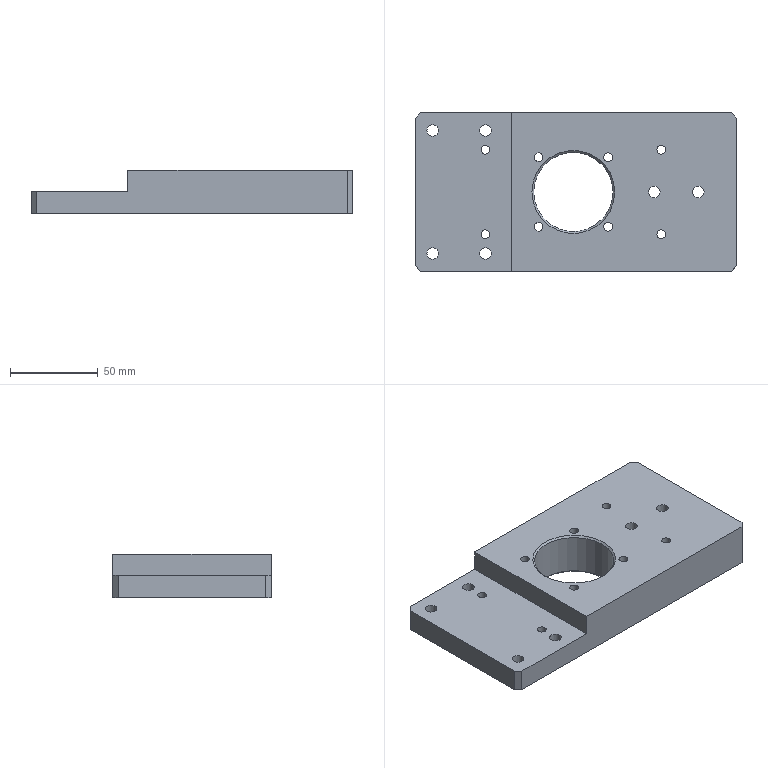Part | 1 solid | 47 faces | box 183 x 90 x 25 mm | volume 301566 mm3 | cylinder 24 | plane 18 | cone 5 | commonest cylinder face diameters 5 x11 6.6 x6 11 x6 45.1 x1
STEP:
#1=CARTESIAN_POINT('',(39.,0.,-5.7));
#2=VERTEX_POINT('',#1);
#3=CARTESIAN_POINT('',(44.5,0.,-5.7));
#4=DIRECTION('',(0.,0.,-1.));
#5=DIRECTION('',(-1.,0.,0.));
#6=AXIS2_PLACEMENT_3D('',#3,#4,#5);
#7=CIRCLE('',#6,5.5);
#8=EDGE_CURVE('',#2,#2,#7,.T.);
#9=ORIENTED_EDGE('',*,*,#8,.T.);
#10=EDGE_LOOP('',(#9));
#11=FACE_BOUND('',#10,.T.);
#12=CARTESIAN_POINT('',(41.2,0.,-5.7));
#13=VERTEX_POINT('',#12);
#14=CARTESIAN_POINT('',(44.5,0.,-5.7));
#15=DIRECTION('',(0.,0.,-1.));
#16=DIRECTION('',(-1.,0.,0.));
#17=AXIS2_PLACEMENT_3D('',#14,#15,#16);
#18=CIRCLE('',#17,3.3);
#19=EDGE_CURVE('',#13,#13,#18,.T.);
#20=ORIENTED_EDGE('',*,*,#19,.F.);
#21=EDGE_LOOP('',(#20));
#22=FACE_BOUND('',#21,.T.);
#23=CARTESIAN_POINT('',(47.8,0.,-5.7));
#24=DIRECTION('',(0.,0.,1.));
#25=DIRECTION('',(1.,0.,0.));
#26=AXIS2_PLACEMENT_3D('',#23,#24,#25);
#27=PLANE('',#26);
#28=ADVANCED_FACE('',(#11,#22),#27,.F.);
#29=CARTESIAN_POINT('',(75.,0.,-5.7));
#30=VERTEX_POINT('',#29);
#31=CARTESIAN_POINT('',(69.5,0.,-5.7));
#32=DIRECTION('',(0.,0.,-1.));
#33=DIRECTION('',(1.,0.,0.));
#34=AXIS2_PLACEMENT_3D('',#31,#32,#33);
#35=CIRCLE('',#34,5.5);
#36=EDGE_CURVE('',#30,#30,#35,.T.);
#37=ORIENTED_EDGE('',*,*,#36,.T.);
#38=EDGE_LOOP('',(#37));
#39=FACE_BOUND('',#38,.T.);
#40=CARTESIAN_POINT('',(72.8,0.,-5.7));
#41=VERTEX_POINT('',#40);
#42=CARTESIAN_POINT('',(69.5,0.,-5.7));
#43=DIRECTION('',(0.,0.,-1.));
#44=DIRECTION('',(1.,0.,0.));
#45=AXIS2_PLACEMENT_3D('',#42,#43,#44);
#46=CIRCLE('',#45,3.3);
#47=EDGE_CURVE('',#41,#41,#46,.T.);
#48=ORIENTED_EDGE('',*,*,#47,.F.);
#49=EDGE_LOOP('',(#48));
#50=FACE_BOUND('',#49,.T.);
#51=CARTESIAN_POINT('',(47.8,0.,-5.7));
#52=DIRECTION('',(0.,0.,1.));
#53=DIRECTION('',(1.,0.,0.));
#54=AXIS2_PLACEMENT_3D('',#51,#52,#53);
#55=PLANE('',#54);
#56=ADVANCED_FACE('',(#39,#50),#55,.F.);
#57=CARTESIAN_POINT('',(-88.5,45.,0.5));
#58=VERTEX_POINT('',#57);
#59=CARTESIAN_POINT('',(-91.5,42.,0.5));
#60=VERTEX_POINT('',#59);
#61=CARTESIAN_POINT('',(-91.5,42.,0.5));
#62=DIRECTION('',(-0.7071,-0.7071,0.));
#63=VECTOR('',#62,1000.);
#64=LINE('',#61,#63);
#65=EDGE_CURVE('',#58,#60,#64,.T.);
#66=ORIENTED_EDGE('',*,*,#65,.F.);
#67=CARTESIAN_POINT('',(-88.5,45.,-12.5));
#68=VERTEX_POINT('',#67);
#69=CARTESIAN_POINT('',(-88.5,45.,12.5));
#70=DIRECTION('',(0.,0.,1.));
#71=VECTOR('',#70,1000.);
#72=LINE('',#69,#71);
#73=EDGE_CURVE('',#68,#58,#72,.T.);
#74=ORIENTED_EDGE('',*,*,#73,.F.);
#75=CARTESIAN_POINT('',(-91.5,42.,-12.5));
#76=VERTEX_POINT('',#75);
#77=CARTESIAN_POINT('',(-91.5,42.,-12.5));
#78=DIRECTION('',(0.7071,0.7071,0.));
#79=VECTOR('',#78,1000.);
#80=LINE('',#77,#79);
#81=EDGE_CURVE('',#76,#68,#80,.T.);
#82=ORIENTED_EDGE('',*,*,#81,.F.);
#83=CARTESIAN_POINT('',(-91.5,42.,12.5));
#84=DIRECTION('',(0.,0.,-1.));
#85=VECTOR('',#84,1000.);
#86=LINE('',#83,#85);
#87=EDGE_CURVE('',#60,#76,#86,.T.);
#88=ORIENTED_EDGE('',*,*,#87,.F.);
#89=EDGE_LOOP('',(#66,#74,#82,#88));
#90=FACE_BOUND('',#89,.T.);
#91=CARTESIAN_POINT('',(-91.5,42.,12.5));
#92=DIRECTION('',(0.7071,-0.7071,0.));
#93=DIRECTION('',(0.,0.,-1.));
#94=AXIS2_PLACEMENT_3D('',#91,#92,#93);
#95=PLANE('',#94);
#96=ADVANCED_FACE('',(#90),#95,.F.);
#97=CARTESIAN_POINT('',(91.5,42.,12.5));
#98=VERTEX_POINT('',#97);
#99=CARTESIAN_POINT('',(88.5,45.,12.5));
#100=VERTEX_POINT('',#99);
#101=CARTESIAN_POINT('',(66.75,66.75,12.5));
#102=DIRECTION('',(-0.7071,0.7071,0.));
#103=VECTOR('',#102,1000.);
#104=LINE('',#101,#103);
#105=EDGE_CURVE('',#98,#100,#104,.T.);
#106=ORIENTED_EDGE('',*,*,#105,.F.);
#107=CARTESIAN_POINT('',(91.5,42.,-12.5));
#108=VERTEX_POINT('',#107);
#109=CARTESIAN_POINT('',(91.5,42.,12.5));
#110=DIRECTION('',(0.,0.,1.));
#111=VECTOR('',#110,1000.);
#112=LINE('',#109,#111);
#113=EDGE_CURVE('',#108,#98,#112,.T.);
#114=ORIENTED_EDGE('',*,*,#113,.F.);
#115=CARTESIAN_POINT('',(88.5,45.,-12.5));
#116=VERTEX_POINT('',#115);
#117=CARTESIAN_POINT('',(88.5,45.,-12.5));
#118=DIRECTION('',(0.7071,-0.7071,0.));
#119=VECTOR('',#118,1000.);
#120=LINE('',#117,#119);
#121=EDGE_CURVE('',#116,#108,#120,.T.);
#122=ORIENTED_EDGE('',*,*,#121,.F.);
#123=CARTESIAN_POINT('',(88.5,45.,12.5));
#124=DIRECTION('',(0.,0.,-1.));
#125=VECTOR('',#124,1000.);
#126=LINE('',#123,#125);
#127=EDGE_CURVE('',#100,#116,#126,.T.);
#128=ORIENTED_EDGE('',*,*,#127,.F.);
#129=EDGE_LOOP('',(#106,#114,#122,#128));
#130=FACE_BOUND('',#129,.T.);
#131=CARTESIAN_POINT('',(88.5,45.,12.5));
#132=DIRECTION('',(-0.7071,-0.7071,0.));
#133=DIRECTION('',(0.,0.,-1.));
#134=AXIS2_PLACEMENT_3D('',#131,#132,#133);
#135=PLANE('',#134);
#136=ADVANCED_FACE('',(#130),#135,.F.);
#137=CARTESIAN_POINT('',(88.5,-45.,12.5));
#138=VERTEX_POINT('',#137);
#139=CARTESIAN_POINT('',(91.5,-42.,12.5));
#140=VERTEX_POINT('',#139);
#141=CARTESIAN_POINT('',(66.75,-66.75,12.5));
#142=DIRECTION('',(0.7071,0.7071,0.));
#143=VECTOR('',#142,1000.);
#144=LINE('',#141,#143);
#145=EDGE_CURVE('',#138,#140,#144,.T.);
#146=ORIENTED_EDGE('',*,*,#145,.F.);
#147=CARTESIAN_POINT('',(88.5,-45.,-12.5));
#148=VERTEX_POINT('',#147);
#149=CARTESIAN_POINT('',(88.5,-45.,12.5));
#150=DIRECTION('',(0.,0.,1.));
#151=VECTOR('',#150,1000.);
#152=LINE('',#149,#151);
#153=EDGE_CURVE('',#148,#138,#152,.T.);
#154=ORIENTED_EDGE('',*,*,#153,.F.);
#155=CARTESIAN_POINT('',(91.5,-42.,-12.5));
#156=VERTEX_POINT('',#155);
#157=CARTESIAN_POINT('',(91.5,-42.,-12.5));
#158=DIRECTION('',(-0.7071,-0.7071,0.));
#159=VECTOR('',#158,1000.);
#160=LINE('',#157,#159);
#161=EDGE_CURVE('',#156,#148,#160,.T.);
#162=ORIENTED_EDGE('',*,*,#161,.F.);
#163=CARTESIAN_POINT('',(91.5,-42.,12.5));
#164=DIRECTION('',(0.,0.,-1.));
#165=VECTOR('',#164,1000.);
#166=LINE('',#163,#165);
#167=EDGE_CURVE('',#140,#156,#166,.T.);
#168=ORIENTED_EDGE('',*,*,#167,.F.);
#169=EDGE_LOOP('',(#146,#154,#162,#168));
#170=FACE_BOUND('',#169,.T.);
#171=CARTESIAN_POINT('',(91.5,-42.,12.5));
#172=DIRECTION('',(-0.7071,0.7071,0.));
#173=DIRECTION('',(0.,0.,-1.));
#174=AXIS2_PLACEMENT_3D('',#171,#172,#173);
#175=PLANE('',#174);
#176=ADVANCED_FACE('',(#170),#175,.F.);
#177=CARTESIAN_POINT('',(-91.5,-42.,0.5));
#178=VERTEX_POINT('',#177);
#179=CARTESIAN_POINT('',(-88.5,-45.,0.5));
#180=VERTEX_POINT('',#179);
#181=CARTESIAN_POINT('',(-88.5,-45.,0.5));
#182=DIRECTION('',(0.7071,-0.7071,0.));
#183=VECTOR('',#182,1000.);
#184=LINE('',#181,#183);
#185=EDGE_CURVE('',#178,#180,#184,.T.);
#186=ORIENTED_EDGE('',*,*,#185,.F.);
#187=CARTESIAN_POINT('',(-91.5,-42.,-12.5));
#188=VERTEX_POINT('',#187);
#189=CARTESIAN_POINT('',(-91.5,-42.,12.5));
#190=DIRECTION('',(0.,0.,1.));
#191=VECTOR('',#190,1000.);
#192=LINE('',#189,#191);
#193=EDGE_CURVE('',#188,#178,#192,.T.);
#194=ORIENTED_EDGE('',*,*,#193,.F.);
#195=CARTESIAN_POINT('',(-88.5,-45.,-12.5));
#196=VERTEX_POINT('',#195);
#197=CARTESIAN_POINT('',(-88.5,-45.,-12.5));
#198=DIRECTION('',(-0.7071,0.7071,0.));
#199=VECTOR('',#198,1000.);
#200=LINE('',#197,#199);
#201=EDGE_CURVE('',#196,#188,#200,.T.);
#202=ORIENTED_EDGE('',*,*,#201,.F.);
#203=CARTESIAN_POINT('',(-88.5,-45.,12.5));
#204=DIRECTION('',(0.,0.,-1.));
#205=VECTOR('',#204,1000.);
#206=LINE('',#203,#205);
#207=EDGE_CURVE('',#180,#196,#206,.T.);
#208=ORIENTED_EDGE('',*,*,#207,.F.);
#209=EDGE_LOOP('',(#186,#194,#202,#208));
#210=FACE_BOUND('',#209,.T.);
#211=CARTESIAN_POINT('',(-88.5,-45.,12.5));
#212=DIRECTION('',(0.7071,0.7071,0.));
#213=DIRECTION('',(0.,0.,-1.));
#214=AXIS2_PLACEMENT_3D('',#211,#212,#213);
#215=PLANE('',#214);
#216=ADVANCED_FACE('',(#210),#215,.F.);
#217=CARTESIAN_POINT('',(-76.,35.,-6.1));
#218=VERTEX_POINT('',#217);
#219=CARTESIAN_POINT('',(-81.5,35.,-6.1));
#220=DIRECTION('',(0.,0.,-1.));
#221=DIRECTION('',(1.,0.,0.));
#222=AXIS2_PLACEMENT_3D('',#219,#220,#221);
#223=CIRCLE('',#222,5.5);
#224=EDGE_CURVE('',#218,#218,#223,.T.);
#225=ORIENTED_EDGE('',*,*,#224,.T.);
#226=EDGE_LOOP('',(#225));
#227=FACE_BOUND('',#226,.T.);
#228=CARTESIAN_POINT('',(-78.2,35.,-6.1));
#229=VERTEX_POINT('',#228);
#230=CARTESIAN_POINT('',(-81.5,35.,-6.1));
#231=DIRECTION('',(0.,0.,-1.));
#232=DIRECTION('',(1.,0.,0.));
#233=AXIS2_PLACEMENT_3D('',#230,#231,#232);
#234=CIRCLE('',#233,3.3);
#235=EDGE_CURVE('',#229,#229,#234,.T.);
#236=ORIENTED_EDGE('',*,*,#235,.F.);
#237=EDGE_LOOP('',(#236));
#238=FACE_BOUND('',#237,.T.);
#239=CARTESIAN_POINT('',(-48.2,35.,-6.1));
#240=DIRECTION('',(0.,0.,1.));
#241=DIRECTION('',(1.,0.,0.));
#242=AXIS2_PLACEMENT_3D('',#239,#240,#241);
#243=PLANE('',#242);
#244=ADVANCED_FACE('',(#227,#238),#243,.F.);
#245=CARTESIAN_POINT('',(-57.,35.,-6.1));
#246=VERTEX_POINT('',#245);
#247=CARTESIAN_POINT('',(-51.5,35.,-6.1));
#248=DIRECTION('',(0.,0.,-1.));
#249=DIRECTION('',(-1.,0.,0.));
#250=AXIS2_PLACEMENT_3D('',#247,#248,#249);
#251=CIRCLE('',#250,5.5);
#252=EDGE_CURVE('',#246,#246,#251,.T.);
#253=ORIENTED_EDGE('',*,*,#252,.T.);
#254=EDGE_LOOP('',(#253));
#255=FACE_BOUND('',#254,.T.);
#256=CARTESIAN_POINT('',(-54.8,35.,-6.1));
#257=VERTEX_POINT('',#256);
#258=CARTESIAN_POINT('',(-51.5,35.,-6.1));
#259=DIRECTION('',(0.,0.,-1.));
#260=DIRECTION('',(-1.,0.,0.));
#261=AXIS2_PLACEMENT_3D('',#258,#259,#260);
#262=CIRCLE('',#261,3.3);
#263=EDGE_CURVE('',#257,#257,#262,.T.);
#264=ORIENTED_EDGE('',*,*,#263,.F.);
#265=EDGE_LOOP('',(#264));
#266=FACE_BOUND('',#265,.T.);
#267=CARTESIAN_POINT('',(-48.2,35.,-6.1));
#268=DIRECTION('',(0.,0.,1.));
#269=DIRECTION('',(1.,0.,0.));
#270=AXIS2_PLACEMENT_3D('',#267,#268,#269);
#271=PLANE('',#270);
#272=ADVANCED_FACE('',(#255,#266),#271,.F.);
#273=CARTESIAN_POINT('',(-46.,-35.,-6.1));
#274=VERTEX_POINT('',#273);
#275=CARTESIAN_POINT('',(-51.5,-35.,-6.1));
#276=DIRECTION('',(0.,0.,-1.));
#277=DIRECTION('',(1.,0.,0.));
#278=AXIS2_PLACEMENT_3D('',#275,#276,#277);
#279=CIRCLE('',#278,5.5);
#280=EDGE_CURVE('',#274,#274,#279,.T.);
#281=ORIENTED_EDGE('',*,*,#280,.T.);
#282=EDGE_LOOP('',(#281));
#283=FACE_BOUND('',#282,.T.);
#284=CARTESIAN_POINT('',(-48.2,-35.,-6.1));
#285=VERTEX_POINT('',#284);
#286=CARTESIAN_POINT('',(-51.5,-35.,-6.1));
#287=DIRECTION('',(0.,0.,-1.));
#288=DIRECTION('',(1.,0.,0.));
#289=AXIS2_PLACEMENT_3D('',#286,#287,#288);
#290=CIRCLE('',#289,3.3);
#291=EDGE_CURVE('',#285,#285,#290,.T.);
#292=ORIENTED_EDGE('',*,*,#291,.F.);
#293=EDGE_LOOP('',(#292));
#294=FACE_BOUND('',#293,.T.);
#295=CARTESIAN_POINT('',(-48.2,35.,-6.1));
#296=DIRECTION('',(0.,0.,1.));
#297=DIRECTION('',(1.,0.,0.));
#298=AXIS2_PLACEMENT_3D('',#295,#296,#297);
#299=PLANE('',#298);
#300=ADVANCED_FACE('',(#283,#294),#299,.F.);
#301=CARTESIAN_POINT('',(-76.,-35.,-6.1));
#302=VERTEX_POINT('',#301);
#303=CARTESIAN_POINT('',(-81.5,-35.,-6.1));
#304=DIRECTION('',(0.,0.,-1.));
#305=DIRECTION('',(1.,0.,0.));
#306=AXIS2_PLACEMENT_3D('',#303,#304,#305);
#307=CIRCLE('',#306,5.5);
#308=EDGE_CURVE('',#302,#302,#307,.T.);
#309=ORIENTED_EDGE('',*,*,#308,.T.);
#310=EDGE_LOOP('',(#309));
#311=FACE_BOUND('',#310,.T.);
#312=CARTESIAN_POINT('',(-78.2,-35.,-6.1));
#313=VERTEX_POINT('',#312);
#314=CARTESIAN_POINT('',(-81.5,-35.,-6.1));
#315=DIRECTION('',(0.,0.,-1.));
#316=DIRECTION('',(1.,0.,0.));
#317=AXIS2_PLACEMENT_3D('',#314,#315,#316);
#318=CIRCLE('',#317,3.3);
#319=EDGE_CURVE('',#313,#313,#318,.T.);
#320=ORIENTED_EDGE('',*,*,#319,.F.);
#321=EDGE_LOOP('',(#320));
#322=FACE_BOUND('',#321,.T.);
#323=CARTESIAN_POINT('',(-48.2,35.,-6.1));
#324=DIRECTION('',(0.,0.,1.));
#325=DIRECTION('',(1.,0.,0.));
#326=AXIS2_PLACEMENT_3D('',#323,#324,#325);
#327=PLANE('',#326);
#328=ADVANCED_FACE('',(#311,#322),#327,.F.);
#329=CARTESIAN_POINT('',(-91.5,-45.,0.5));
#330=DIRECTION('',(0.,-1.,0.));
#331=VECTOR('',#330,1000.);
#332=LINE('',#329,#331);
#333=EDGE_CURVE('',#60,#178,#332,.T.);
#334=ORIENTED_EDGE('',*,*,#333,.T.);
#335=ORIENTED_EDGE('',*,*,#185,.T.);
#336=CARTESIAN_POINT('',(-36.5,-45.,0.5));
#337=VERTEX_POINT('',#336);
#338=CARTESIAN_POINT('',(-91.5,-45.,0.5));
#339=DIRECTION('',(1.,0.,0.));
#340=VECTOR('',#339,1000.);
#341=LINE('',#338,#340);
#342=EDGE_CURVE('',#180,#337,#341,.T.);
#343=ORIENTED_EDGE('',*,*,#342,.T.);
#344=CARTESIAN_POINT('',(-36.5,45.,0.5));
#345=VERTEX_POINT('',#344);
#346=CARTESIAN_POINT('',(-36.5,-45.,0.5));
#347=DIRECTION('',(0.,1.,0.));
#348=VECTOR('',#347,1000.);
#349=LINE('',#346,#348);
#350=EDGE_CURVE('',#337,#345,#349,.T.);
#351=ORIENTED_EDGE('',*,*,#350,.T.);
#352=CARTESIAN_POINT('',(-91.5,45.,0.5));
#353=DIRECTION('',(-1.,0.,0.));
#354=VECTOR('',#353,1000.);
#355=LINE('',#352,#354);
#356=EDGE_CURVE('',#345,#58,#355,.T.);
#357=ORIENTED_EDGE('',*,*,#356,.T.);
#358=ORIENTED_EDGE('',*,*,#65,.T.);
#359=EDGE_LOOP('',(#334,#335,#343,#351,#357,#358));
#360=FACE_BOUND('',#359,.T.);
#361=CARTESIAN_POINT('',(-84.8,-35.,0.5));
#362=VERTEX_POINT('',#361);
#363=CARTESIAN_POINT('',(-81.5,-35.,0.5));
#364=DIRECTION('',(0.,0.,-1.));
#365=DIRECTION('',(-1.,0.,0.));
#366=AXIS2_PLACEMENT_3D('',#363,#364,#365);
#367=CIRCLE('',#366,3.3);
#368=EDGE_CURVE('',#362,#362,#367,.T.);
#369=ORIENTED_EDGE('',*,*,#368,.T.);
#370=EDGE_LOOP('',(#369));
#371=FACE_BOUND('',#370,.T.);
#372=CARTESIAN_POINT('',(-54.8,-35.,0.5));
#373=VERTEX_POINT('',#372);
#374=CARTESIAN_POINT('',(-51.5,-35.,0.5));
#375=DIRECTION('',(0.,0.,-1.));
#376=DIRECTION('',(-1.,0.,0.));
#377=AXIS2_PLACEMENT_3D('',#374,#375,#376);
#378=CIRCLE('',#377,3.3);
#379=EDGE_CURVE('',#373,#373,#378,.T.);
#380=ORIENTED_EDGE('',*,*,#379,.T.);
#381=EDGE_LOOP('',(#380));
#382=FACE_BOUND('',#381,.T.);
#383=CARTESIAN_POINT('',(-54.8,35.,0.5));
#384=VERTEX_POINT('',#383);
#385=CARTESIAN_POINT('',(-51.5,35.,0.5));
#386=DIRECTION('',(0.,0.,-1.));
#387=DIRECTION('',(-1.,0.,0.));
#388=AXIS2_PLACEMENT_3D('',#385,#386,#387);
#389=CIRCLE('',#388,3.3);
#390=EDGE_CURVE('',#384,#384,#389,.T.);
#391=ORIENTED_EDGE('',*,*,#390,.T.);
#392=EDGE_LOOP('',(#391));
#393=FACE_BOUND('',#392,.T.);
#394=CARTESIAN_POINT('',(-84.8,35.,0.5));
#395=VERTEX_POINT('',#394);
#396=CARTESIAN_POINT('',(-81.5,35.,0.5));
#397=DIRECTION('',(0.,0.,-1.));
#398=DIRECTION('',(-1.,0.,0.));
#399=AXIS2_PLACEMENT_3D('',#396,#397,#398);
#400=CIRCLE('',#399,3.3);
#401=EDGE_CURVE('',#395,#395,#400,.T.);
#402=ORIENTED_EDGE('',*,*,#401,.T.);
#403=EDGE_LOOP('',(#402));
#404=FACE_BOUND('',#403,.T.);
#405=CARTESIAN_POINT('',(-54.,-24.,0.5));
#406=VERTEX_POINT('',#405);
#407=CARTESIAN_POINT('',(-51.5,-24.,0.5));
#408=DIRECTION('',(0.,0.,-1.));
#409=DIRECTION('',(-1.,0.,0.));
#410=AXIS2_PLACEMENT_3D('',#407,#408,#409);
#411=CIRCLE('',#410,2.5);
#412=EDGE_CURVE('',#406,#406,#411,.T.);
#413=ORIENTED_EDGE('',*,*,#412,.T.);
#414=EDGE_LOOP('',(#413));
#415=FACE_BOUND('',#414,.T.);
#416=CARTESIAN_POINT('',(-54.,24.,0.5));
#417=VERTEX_POINT('',#416);
#418=CARTESIAN_POINT('',(-51.5,24.,0.5));
#419=DIRECTION('',(0.,0.,-1.));
#420=DIRECTION('',(-1.,0.,0.));
#421=AXIS2_PLACEMENT_3D('',#418,#419,#420);
#422=CIRCLE('',#421,2.5);
#423=EDGE_CURVE('',#417,#417,#422,.T.);
#424=ORIENTED_EDGE('',*,*,#423,.T.);
#425=EDGE_LOOP('',(#424));
#426=FACE_BOUND('',#425,.T.);
#427=CARTESIAN_POINT('',(0.,0.,0.5));
#428=DIRECTION('',(0.,0.,-1.));
#429=DIRECTION('',(-1.,0.,0.));
#430=AXIS2_PLACEMENT_3D('',#427,#428,#429);
#431=PLANE('',#430);
#432=ADVANCED_FACE('',(#360,#371,#382,#393,#404,#415,#426),#431,.F.);
#433=CARTESIAN_POINT('',(-36.5,-45.,12.5));
#434=VERTEX_POINT('',#433);
#435=CARTESIAN_POINT('',(-36.5,45.,12.5));
#436=VERTEX_POINT('',#435);
#437=CARTESIAN_POINT('',(-36.5,-45.,12.5));
#438=DIRECTION('',(0.,1.,0.));
#439=VECTOR('',#438,1000.);
#440=LINE('',#437,#439);
#441=EDGE_CURVE('',#434,#436,#440,.T.);
#442=ORIENTED_EDGE('',*,*,#441,.T.);
#443=CARTESIAN_POINT('',(-36.5,45.,0.5));
#444=DIRECTION('',(0.,0.,1.));
#445=VECTOR('',#444,1000.);
#446=LINE('',#443,#445);
#447=EDGE_CURVE('',#345,#436,#446,.T.);
#448=ORIENTED_EDGE('',*,*,#447,.F.);
#449=ORIENTED_EDGE('',*,*,#350,.F.);
#450=CARTESIAN_POINT('',(-36.5,-45.,0.5));
#451=DIRECTION('',(0.,0.,1.));
#452=VECTOR('',#451,1000.);
#453=LINE('',#450,#452);
#454=EDGE_CURVE('',#337,#434,#453,.T.);
#455=ORIENTED_EDGE('',*,*,#454,.T.);
#456=EDGE_LOOP('',(#442,#448,#449,#455));
#457=FACE_BOUND('',#456,.T.);
#458=CARTESIAN_POINT('',(-36.5,-45.,0.5));
#459=DIRECTION('',(1.,0.,0.));
#460=DIRECTION('',(0.,1.,0.));
#461=AXIS2_PLACEMENT_3D('',#458,#459,#460);
#462=PLANE('',#461);
#463=ADVANCED_FACE('',(#457),#462,.F.);
#464=CARTESIAN_POINT('',(-91.5,-45.,-12.5));
#465=DIRECTION('',(1.,0.,0.));
#466=VECTOR('',#465,1000.);
#467=LINE('',#464,#466);
#468=EDGE_CURVE('',#196,#148,#467,.T.);
#469=ORIENTED_EDGE('',*,*,#468,.F.);
#470=ORIENTED_EDGE('',*,*,#201,.T.);
#471=CARTESIAN_POINT('',(-91.5,45.,-12.5));
#472=DIRECTION('',(0.,-1.,0.));
#473=VECTOR('',#472,1000.);
#474=LINE('',#471,#473);
#475=EDGE_CURVE('',#76,#188,#474,.T.);
#476=ORIENTED_EDGE('',*,*,#475,.F.);
#477=ORIENTED_EDGE('',*,*,#81,.T.);
#478=CARTESIAN_POINT('',(-91.5,45.,-12.5));
#479=DIRECTION('',(-1.,0.,0.));
#480=VECTOR('',#479,1000.);
#481=LINE('',#478,#480);
#482=EDGE_CURVE('',#116,#68,#481,.T.);
#483=ORIENTED_EDGE('',*,*,#482,.F.);
#484=ORIENTED_EDGE('',*,*,#121,.T.);
#485=CARTESIAN_POINT('',(91.5,45.,-12.5));
#486=DIRECTION('',(0.,1.,0.));
#487=VECTOR('',#486,1000.);
#488=LINE('',#485,#487);
#489=EDGE_CURVE('',#156,#108,#488,.T.);
#490=ORIENTED_EDGE('',*,*,#489,.F.);
#491=ORIENTED_EDGE('',*,*,#161,.T.);
#492=EDGE_LOOP('',(#469,#470,#476,#477,#483,#484,#490,#491));
#493=FACE_BOUND('',#492,.T.);
#494=CARTESIAN_POINT('',(-87.,-35.,-12.5));
#495=VERTEX_POINT('',#494);
#496=CARTESIAN_POINT('',(-81.5,-35.,-12.5));
#497=DIRECTION('',(0.,0.,-1.));
#498=DIRECTION('',(-1.,0.,0.));
#499=AXIS2_PLACEMENT_3D('',#496,#497,#498);
#500=CIRCLE('',#499,5.5);
#501=EDGE_CURVE('',#495,#495,#500,.T.);
#502=ORIENTED_EDGE('',*,*,#501,.F.);
#503=EDGE_LOOP('',(#502));
#504=FACE_BOUND('',#503,.T.);
#505=CARTESIAN_POINT('',(-57.,-35.,-12.5));
#506=VERTEX_POINT('',#505);
#507=CARTESIAN_POINT('',(-51.5,-35.,-12.5));
#508=DIRECTION('',(0.,0.,-1.));
#509=DIRECTION('',(-1.,0.,0.));
#510=AXIS2_PLACEMENT_3D('',#507,#508,#509);
#511=CIRCLE('',#510,5.5);
#512=EDGE_CURVE('',#506,#506,#511,.T.);
#513=ORIENTED_EDGE('',*,*,#512,.F.);
#514=EDGE_LOOP('',(#513));
#515=FACE_BOUND('',#514,.T.);
#516=CARTESIAN_POINT('',(-57.,35.,-12.5));
#517=VERTEX_POINT('',#516);
#518=CARTESIAN_POINT('',(-51.5,35.,-12.5));
#519=DIRECTION('',(0.,0.,-1.));
#520=DIRECTION('',(-1.,0.,0.));
#521=AXIS2_PLACEMENT_3D('',#518,#519,#520);
#522=CIRCLE('',#521,5.5);
#523=EDGE_CURVE('',#517,#517,#522,.T.);
#524=ORIENTED_EDGE('',*,*,#523,.F.);
#525=EDGE_LOOP('',(#524));
#526=FACE_BOUND('',#525,.T.);
#527=CARTESIAN_POINT('',(-87.,35.,-12.5));
#528=VERTEX_POINT('',#527);
#529=CARTESIAN_POINT('',(-81.5,35.,-12.5));
#530=DIRECTION('',(0.,0.,-1.));
#531=DIRECTION('',(-1.,0.,0.));
#532=AXIS2_PLACEMENT_3D('',#529,#530,#531);
#533=CIRCLE('',#532,5.5);
#534=EDGE_CURVE('',#528,#528,#533,.T.);
#535=ORIENTED_EDGE('',*,*,#534,.F.);
#536=EDGE_LOOP('',(#535));
#537=FACE_BOUND('',#536,.T.);
#538=CARTESIAN_POINT('',(22.05,0.,-12.5));
#539=VERTEX_POINT('',#538);
#540=CARTESIAN_POINT('',(-1.5,0.,-12.5));
#541=DIRECTION('',(0.,0.,1.));
#542=DIRECTION('',(1.,0.,0.));
#543=AXIS2_PLACEMENT_3D('',#540,#541,#542);
#544=CIRCLE('',#543,23.55);
#545=EDGE_CURVE('',#539,#539,#544,.T.);
#546=ORIENTED_EDGE('',*,*,#545,.T.);
#547=EDGE_LOOP('',(#546));
#548=FACE_BOUND('',#547,.T.);
#549=CARTESIAN_POINT('',(15.799,-19.799,-12.5));
#550=VERTEX_POINT('',#549);
#551=CARTESIAN_POINT('',(18.299,-19.799,-12.5));
#552=DIRECTION('',(0.,0.,-1.));
#553=DIRECTION('',(-1.,0.,0.));
#554=AXIS2_PLACEMENT_3D('',#551,#552,#553);
#555=CIRCLE('',#554,2.5);
#556=EDGE_CURVE('',#550,#550,#555,.T.);
#557=ORIENTED_EDGE('',*,*,#556,.F.);
#558=EDGE_LOOP('',(#557));
#559=FACE_BOUND('',#558,.T.);
#560=CARTESIAN_POINT('',(-23.799,-19.799,-12.5));
#561=VERTEX_POINT('',#560);
#562=CARTESIAN_POINT('',(-21.299,-19.799,-12.5));
#563=DIRECTION('',(0.,0.,-1.));
#564=DIRECTION('',(-1.,0.,0.));
#565=AXIS2_PLACEMENT_3D('',#562,#563,#564);
#566=CIRCLE('',#565,2.5);
#567=EDGE_CURVE('',#561,#561,#566,.T.);
#568=ORIENTED_EDGE('',*,*,#567,.F.);
#569=EDGE_LOOP('',(#568));
#570=FACE_BOUND('',#569,.T.);
#571=CARTESIAN_POINT('',(-23.799,19.799,-12.5));
#572=VERTEX_POINT('',#571);
#573=CARTESIAN_POINT('',(-21.299,19.799,-12.5));
#574=DIRECTION('',(0.,0.,-1.));
#575=DIRECTION('',(-1.,0.,0.));
#576=AXIS2_PLACEMENT_3D('',#573,#574,#575);
#577=CIRCLE('',#576,2.5);
#578=EDGE_CURVE('',#572,#572,#577,.T.);
#579=ORIENTED_EDGE('',*,*,#578,.F.);
#580=EDGE_LOOP('',(#579));
#581=FACE_BOUND('',#580,.T.);
#582=CARTESIAN_POINT('',(15.799,19.799,-12.5));
#583=VERTEX_POINT('',#582);
#584=CARTESIAN_POINT('',(18.299,19.799,-12.5));
#585=DIRECTION('',(0.,0.,-1.));
#586=DIRECTION('',(-1.,0.,0.));
#587=AXIS2_PLACEMENT_3D('',#584,#585,#586);
#588=CIRCLE('',#587,2.5);
#589=EDGE_CURVE('',#583,#583,#588,.T.);
#590=ORIENTED_EDGE('',*,*,#589,.F.);
#591=EDGE_LOOP('',(#590));
#592=FACE_BOUND('',#591,.T.);
#593=CARTESIAN_POINT('',(64.,0.,-12.5));
#594=VERTEX_POINT('',#593);
#595=CARTESIAN_POINT('',(69.5,0.,-12.5));
#596=DIRECTION('',(0.,0.,-1.));
#597=DIRECTION('',(-1.,0.,0.));
#598=AXIS2_PLACEMENT_3D('',#595,#596,#597);
#599=CIRCLE('',#598,5.5);
#600=EDGE_CURVE('',#594,#594,#599,.T.);
#601=ORIENTED_EDGE('',*,*,#600,.F.);
#602=EDGE_LOOP('',(#601));
#603=FACE_BOUND('',#602,.T.);
#604=CARTESIAN_POINT('',(39.,0.,-12.5));
#605=VERTEX_POINT('',#604);
#606=CARTESIAN_POINT('',(44.5,0.,-12.5));
#607=DIRECTION('',(0.,0.,-1.));
#608=DIRECTION('',(-1.,0.,0.));
#609=AXIS2_PLACEMENT_3D('',#606,#607,#608);
#610=CIRCLE('',#609,5.5);
#611=EDGE_CURVE('',#605,#605,#610,.T.);
#612=ORIENTED_EDGE('',*,*,#611,.F.);
#613=EDGE_LOOP('',(#612));
#614=FACE_BOUND('',#613,.T.);
#615=CARTESIAN_POINT('',(46.,24.,-12.5));
#616=VERTEX_POINT('',#615);
#617=CARTESIAN_POINT('',(48.5,24.,-12.5));
#618=DIRECTION('',(0.,0.,-1.));
#619=DIRECTION('',(-1.,0.,0.));
#620=AXIS2_PLACEMENT_3D('',#617,#618,#619);
#621=CIRCLE('',#620,2.5);
#622=EDGE_CURVE('',#616,#616,#621,.T.);
#623=ORIENTED_EDGE('',*,*,#622,.F.);
#624=EDGE_LOOP('',(#623));
#625=FACE_BOUND('',#624,.T.);
#626=CARTESIAN_POINT('',(46.,-24.,-12.5));
#627=VERTEX_POINT('',#626);
#628=CARTESIAN_POINT('',(48.5,-24.,-12.5));
#629=DIRECTION('',(0.,0.,-1.));
#630=DIRECTION('',(-1.,0.,0.));
#631=AXIS2_PLACEMENT_3D('',#628,#629,#630);
#632=CIRCLE('',#631,2.5);
#633=EDGE_CURVE('',#627,#627,#632,.T.);
#634=ORIENTED_EDGE('',*,*,#633,.F.);
#635=EDGE_LOOP('',(#634));
#636=FACE_BOUND('',#635,.T.);
#637=CARTESIAN_POINT('',(-54.,-24.,-12.5));
#638=VERTEX_POINT('',#637);
#639=CARTESIAN_POINT('',(-51.5,-24.,-12.5));
#640=DIRECTION('',(0.,0.,-1.));
#641=DIRECTION('',(-1.,0.,0.));
#642=AXIS2_PLACEMENT_3D('',#639,#640,#641);
#643=CIRCLE('',#642,2.5);
#644=EDGE_CURVE('',#638,#638,#643,.T.);
#645=ORIENTED_EDGE('',*,*,#644,.F.);
#646=EDGE_LOOP('',(#645));
#647=FACE_BOUND('',#646,.T.);
#648=CARTESIAN_POINT('',(-54.,24.,-12.5));
#649=VERTEX_POINT('',#648);
#650=CARTESIAN_POINT('',(-51.5,24.,-12.5));
#651=DIRECTION('',(0.,0.,-1.));
#652=DIRECTION('',(-1.,0.,0.));
#653=AXIS2_PLACEMENT_3D('',#650,#651,#652);
#654=CIRCLE('',#653,2.5);
#655=EDGE_CURVE('',#649,#649,#654,.T.);
#656=ORIENTED_EDGE('',*,*,#655,.F.);
#657=EDGE_LOOP('',(#656));
#658=FACE_BOUND('',#657,.T.);
#659=CARTESIAN_POINT('',(0.,0.,-12.5));
#660=DIRECTION('',(0.,0.,1.));
#661=DIRECTION('',(1.,0.,0.));
#662=AXIS2_PLACEMENT_3D('',#659,#660,#661);
#663=PLANE('',#662);
#664=ADVANCED_FACE('',(#493,#504,#515,#526,#537,#548,#559,#570,#581,#592,#603,#614,#625,#636,#647,#658),#663,.F.);
#665=CARTESIAN_POINT('',(-91.5,-45.,12.5));
#666=DIRECTION('',(1.,0.,0.));
#667=VECTOR('',#666,1000.);
#668=LINE('',#665,#667);
#669=EDGE_CURVE('',#434,#138,#668,.T.);
#670=ORIENTED_EDGE('',*,*,#669,.T.);
#671=ORIENTED_EDGE('',*,*,#145,.T.);
#672=CARTESIAN_POINT('',(91.5,45.,12.5));
#673=DIRECTION('',(0.,1.,0.));
#674=VECTOR('',#673,1000.);
#675=LINE('',#672,#674);
#676=EDGE_CURVE('',#140,#98,#675,.T.);
#677=ORIENTED_EDGE('',*,*,#676,.T.);
#678=ORIENTED_EDGE('',*,*,#105,.T.);
#679=CARTESIAN_POINT('',(-91.5,45.,12.5));
#680=DIRECTION('',(-1.,0.,0.));
#681=VECTOR('',#680,1000.);
#682=LINE('',#679,#681);
#683=EDGE_CURVE('',#100,#436,#682,.T.);
#684=ORIENTED_EDGE('',*,*,#683,.T.);
#685=ORIENTED_EDGE('',*,*,#441,.F.);
#686=EDGE_LOOP('',(#670,#671,#677,#678,#684,#685));
#687=FACE_BOUND('',#686,.T.);
#688=CARTESIAN_POINT('',(22.05,0.,12.5));
#689=VERTEX_POINT('',#688);
#690=CARTESIAN_POINT('',(-1.5,0.,12.5));
#691=DIRECTION('',(0.,0.,-1.));
#692=DIRECTION('',(1.,0.,0.));
#693=AXIS2_PLACEMENT_3D('',#690,#691,#692);
#694=CIRCLE('',#693,23.55);
#695=EDGE_CURVE('',#689,#689,#694,.T.);
#696=ORIENTED_EDGE('',*,*,#695,.T.);
#697=EDGE_LOOP('',(#696));
#698=FACE_BOUND('',#697,.T.);
#699=CARTESIAN_POINT('',(15.799,-19.799,12.5));
#700=VERTEX_POINT('',#699);
#701=CARTESIAN_POINT('',(18.299,-19.799,12.5));
#702=DIRECTION('',(0.,0.,-1.));
#703=DIRECTION('',(-1.,0.,0.));
#704=AXIS2_PLACEMENT_3D('',#701,#702,#703);
#705=CIRCLE('',#704,2.5);
#706=EDGE_CURVE('',#700,#700,#705,.T.);
#707=ORIENTED_EDGE('',*,*,#706,.T.);
#708=EDGE_LOOP('',(#707));
#709=FACE_BOUND('',#708,.T.);
#710=CARTESIAN_POINT('',(-23.799,-19.799,12.5));
#711=VERTEX_POINT('',#710);
#712=CARTESIAN_POINT('',(-21.299,-19.799,12.5));
#713=DIRECTION('',(0.,0.,-1.));
#714=DIRECTION('',(-1.,0.,0.));
#715=AXIS2_PLACEMENT_3D('',#712,#713,#714);
#716=CIRCLE('',#715,2.5);
#717=EDGE_CURVE('',#711,#711,#716,.T.);
#718=ORIENTED_EDGE('',*,*,#717,.T.);
#719=EDGE_LOOP('',(#718));
#720=FACE_BOUND('',#719,.T.);
#721=CARTESIAN_POINT('',(-23.799,19.799,12.5));
#722=VERTEX_POINT('',#721);
#723=CARTESIAN_POINT('',(-21.299,19.799,12.5));
#724=DIRECTION('',(0.,0.,-1.));
#725=DIRECTION('',(-1.,0.,0.));
#726=AXIS2_PLACEMENT_3D('',#723,#724,#725);
#727=CIRCLE('',#726,2.5);
#728=EDGE_CURVE('',#722,#722,#727,.T.);
#729=ORIENTED_EDGE('',*,*,#728,.T.);
#730=EDGE_LOOP('',(#729));
#731=FACE_BOUND('',#730,.T.);
#732=CARTESIAN_POINT('',(15.799,19.799,12.5));
#733=VERTEX_POINT('',#732);
#734=CARTESIAN_POINT('',(18.299,19.799,12.5));
#735=DIRECTION('',(0.,0.,-1.));
#736=DIRECTION('',(-1.,0.,0.));
#737=AXIS2_PLACEMENT_3D('',#734,#735,#736);
#738=CIRCLE('',#737,2.5);
#739=EDGE_CURVE('',#733,#733,#738,.T.);
#740=ORIENTED_EDGE('',*,*,#739,.T.);
#741=EDGE_LOOP('',(#740));
#742=FACE_BOUND('',#741,.T.);
#743=CARTESIAN_POINT('',(66.2,0.,12.5));
#744=VERTEX_POINT('',#743);
#745=CARTESIAN_POINT('',(69.5,0.,12.5));
#746=DIRECTION('',(0.,0.,-1.));
#747=DIRECTION('',(-1.,0.,0.));
#748=AXIS2_PLACEMENT_3D('',#745,#746,#747);
#749=CIRCLE('',#748,3.3);
#750=EDGE_CURVE('',#744,#744,#749,.T.);
#751=ORIENTED_EDGE('',*,*,#750,.T.);
#752=EDGE_LOOP('',(#751));
#753=FACE_BOUND('',#752,.T.);
#754=CARTESIAN_POINT('',(41.2,0.,12.5));
#755=VERTEX_POINT('',#754);
#756=CARTESIAN_POINT('',(44.5,0.,12.5));
#757=DIRECTION('',(0.,0.,-1.));
#758=DIRECTION('',(-1.,0.,0.));
#759=AXIS2_PLACEMENT_3D('',#756,#757,#758);
#760=CIRCLE('',#759,3.3);
#761=EDGE_CURVE('',#755,#755,#760,.T.);
#762=ORIENTED_EDGE('',*,*,#761,.T.);
#763=EDGE_LOOP('',(#762));
#764=FACE_BOUND('',#763,.T.);
#765=CARTESIAN_POINT('',(46.,24.,12.5));
#766=VERTEX_POINT('',#765);
#767=CARTESIAN_POINT('',(48.5,24.,12.5));
#768=DIRECTION('',(0.,0.,-1.));
#769=DIRECTION('',(-1.,0.,0.));
#770=AXIS2_PLACEMENT_3D('',#767,#768,#769);
#771=CIRCLE('',#770,2.5);
#772=EDGE_CURVE('',#766,#766,#771,.T.);
#773=ORIENTED_EDGE('',*,*,#772,.T.);
#774=EDGE_LOOP('',(#773));
#775=FACE_BOUND('',#774,.T.);
#776=CARTESIAN_POINT('',(46.,-24.,12.5));
#777=VERTEX_POINT('',#776);
#778=CARTESIAN_POINT('',(48.5,-24.,12.5));
#779=DIRECTION('',(0.,0.,-1.));
#780=DIRECTION('',(-1.,0.,0.));
#781=AXIS2_PLACEMENT_3D('',#778,#779,#780);
#782=CIRCLE('',#781,2.5);
#783=EDGE_CURVE('',#777,#777,#782,.T.);
#784=ORIENTED_EDGE('',*,*,#783,.T.);
#785=EDGE_LOOP('',(#784));
#786=FACE_BOUND('',#785,.T.);
#787=CARTESIAN_POINT('',(0.,0.,12.5));
#788=DIRECTION('',(0.,0.,1.));
#789=DIRECTION('',(1.,0.,0.));
#790=AXIS2_PLACEMENT_3D('',#787,#788,#789);
#791=PLANE('',#790);
#792=ADVANCED_FACE('',(#687,#698,#709,#720,#731,#742,#753,#764,#775,#786),#791,.T.);
#793=ORIENTED_EDGE('',*,*,#342,.F.);
#794=ORIENTED_EDGE('',*,*,#207,.T.);
#795=ORIENTED_EDGE('',*,*,#468,.T.);
#796=ORIENTED_EDGE('',*,*,#153,.T.);
#797=ORIENTED_EDGE('',*,*,#669,.F.);
#798=ORIENTED_EDGE('',*,*,#454,.F.);
#799=EDGE_LOOP('',(#793,#794,#795,#796,#797,#798));
#800=FACE_BOUND('',#799,.T.);
#801=CARTESIAN_POINT('',(-91.5,-45.,12.5));
#802=DIRECTION('',(0.,1.,0.));
#803=DIRECTION('',(0.,0.,1.));
#804=AXIS2_PLACEMENT_3D('',#801,#802,#803);
#805=PLANE('',#804);
#806=ADVANCED_FACE('',(#800),#805,.F.);
#807=ORIENTED_EDGE('',*,*,#475,.T.);
#808=ORIENTED_EDGE('',*,*,#193,.T.);
#809=ORIENTED_EDGE('',*,*,#333,.F.);
#810=ORIENTED_EDGE('',*,*,#87,.T.);
#811=EDGE_LOOP('',(#807,#808,#809,#810));
#812=FACE_BOUND('',#811,.T.);
#813=CARTESIAN_POINT('',(-91.5,45.,12.5));
#814=DIRECTION('',(1.,0.,0.));
#815=DIRECTION('',(0.,0.,-1.));
#816=AXIS2_PLACEMENT_3D('',#813,#814,#815);
#817=PLANE('',#816);
#818=ADVANCED_FACE('',(#812),#817,.F.);
#819=ORIENTED_EDGE('',*,*,#683,.F.);
#820=ORIENTED_EDGE('',*,*,#127,.T.);
#821=ORIENTED_EDGE('',*,*,#482,.T.);
#822=ORIENTED_EDGE('',*,*,#73,.T.);
#823=ORIENTED_EDGE('',*,*,#356,.F.);
#824=ORIENTED_EDGE('',*,*,#447,.T.);
#825=EDGE_LOOP('',(#819,#820,#821,#822,#823,#824));
#826=FACE_BOUND('',#825,.T.);
#827=CARTESIAN_POINT('',(-91.5,45.,12.5));
#828=DIRECTION('',(0.,-1.,0.));
#829=DIRECTION('',(1.,0.,0.));
#830=AXIS2_PLACEMENT_3D('',#827,#828,#829);
#831=PLANE('',#830);
#832=ADVANCED_FACE('',(#826),#831,.F.);
#833=ORIENTED_EDGE('',*,*,#676,.F.);
#834=ORIENTED_EDGE('',*,*,#167,.T.);
#835=ORIENTED_EDGE('',*,*,#489,.T.);
#836=ORIENTED_EDGE('',*,*,#113,.T.);
#837=EDGE_LOOP('',(#833,#834,#835,#836));
#838=FACE_BOUND('',#837,.T.);
#839=CARTESIAN_POINT('',(91.5,-35.,-2.5));
#840=VERTEX_POINT('',#839);
#841=CARTESIAN_POINT('',(91.5,-35.,0.));
#842=DIRECTION('',(1.,0.,0.));
#843=DIRECTION('',(0.,0.,-1.));
#844=AXIS2_PLACEMENT_3D('',#841,#842,#843);
#845=CIRCLE('',#844,2.5);
#846=EDGE_CURVE('',#840,#840,#845,.T.);
#847=ORIENTED_EDGE('',*,*,#846,.F.);
#848=EDGE_LOOP('',(#847));
#849=FACE_BOUND('',#848,.T.);
#850=CARTESIAN_POINT('',(91.5,0.,-2.5));
#851=VERTEX_POINT('',#850);
#852=CARTESIAN_POINT('',(91.5,0.,0.));
#853=DIRECTION('',(1.,0.,0.));
#854=DIRECTION('',(0.,0.,-1.));
#855=AXIS2_PLACEMENT_3D('',#852,#853,#854);
#856=CIRCLE('',#855,2.5);
#857=EDGE_CURVE('',#851,#851,#856,.T.);
#858=ORIENTED_EDGE('',*,*,#857,.F.);
#859=EDGE_LOOP('',(#858));
#860=FACE_BOUND('',#859,.T.);
#861=CARTESIAN_POINT('',(91.5,35.,-2.5));
#862=VERTEX_POINT('',#861);
#863=CARTESIAN_POINT('',(91.5,35.,0.));
#864=DIRECTION('',(1.,0.,0.));
#865=DIRECTION('',(0.,0.,-1.));
#866=AXIS2_PLACEMENT_3D('',#863,#864,#865);
#867=CIRCLE('',#866,2.5);
#868=EDGE_CURVE('',#862,#862,#867,.T.);
#869=ORIENTED_EDGE('',*,*,#868,.F.);
#870=EDGE_LOOP('',(#869));
#871=FACE_BOUND('',#870,.T.);
#872=CARTESIAN_POINT('',(91.5,45.,12.5));
#873=DIRECTION('',(-1.,0.,0.));
#874=DIRECTION('',(0.,0.,1.));
#875=AXIS2_PLACEMENT_3D('',#872,#873,#874);
#876=PLANE('',#875);
#877=ADVANCED_FACE('',(#838,#849,#860,#871),#876,.F.);
#878=ORIENTED_EDGE('',*,*,#319,.T.);
#879=EDGE_LOOP('',(#878));
#880=FACE_BOUND('',#879,.T.);
#881=ORIENTED_EDGE('',*,*,#368,.F.);
#882=EDGE_LOOP('',(#881));
#883=FACE_BOUND('',#882,.T.);
#884=CARTESIAN_POINT('',(-81.5,-35.,-12.5));
#885=DIRECTION('',(0.,0.,-1.));
#886=DIRECTION('',(-1.,0.,0.));
#887=AXIS2_PLACEMENT_3D('',#884,#885,#886);
#888=CYLINDRICAL_SURFACE('',#887,3.3);
#889=ADVANCED_FACE('',(#880,#883),#888,.F.);
#890=ORIENTED_EDGE('',*,*,#501,.T.);
#891=EDGE_LOOP('',(#890));
#892=FACE_BOUND('',#891,.T.);
#893=ORIENTED_EDGE('',*,*,#308,.F.);
#894=EDGE_LOOP('',(#893));
#895=FACE_BOUND('',#894,.T.);
#896=CARTESIAN_POINT('',(-81.5,-35.,-12.5));
#897=DIRECTION('',(0.,0.,-1.));
#898=DIRECTION('',(-1.,0.,0.));
#899=AXIS2_PLACEMENT_3D('',#896,#897,#898);
#900=CYLINDRICAL_SURFACE('',#899,5.5);
#901=ADVANCED_FACE('',(#892,#895),#900,.F.);
#902=ORIENTED_EDGE('',*,*,#291,.T.);
#903=EDGE_LOOP('',(#902));
#904=FACE_BOUND('',#903,.T.);
#905=ORIENTED_EDGE('',*,*,#379,.F.);
#906=EDGE_LOOP('',(#905));
#907=FACE_BOUND('',#906,.T.);
#908=CARTESIAN_POINT('',(-51.5,-35.,-12.5));
#909=DIRECTION('',(0.,0.,-1.));
#910=DIRECTION('',(-1.,0.,0.));
#911=AXIS2_PLACEMENT_3D('',#908,#909,#910);
#912=CYLINDRICAL_SURFACE('',#911,3.3);
#913=ADVANCED_FACE('',(#904,#907),#912,.F.);
#914=ORIENTED_EDGE('',*,*,#512,.T.);
#915=EDGE_LOOP('',(#914));
#916=FACE_BOUND('',#915,.T.);
#917=ORIENTED_EDGE('',*,*,#280,.F.);
#918=EDGE_LOOP('',(#917));
#919=FACE_BOUND('',#918,.T.);
#920=CARTESIAN_POINT('',(-51.5,-35.,-12.5));
#921=DIRECTION('',(0.,0.,-1.));
#922=DIRECTION('',(-1.,0.,0.));
#923=AXIS2_PLACEMENT_3D('',#920,#921,#922);
#924=CYLINDRICAL_SURFACE('',#923,5.5);
#925=ADVANCED_FACE('',(#916,#919),#924,.F.);
#926=ORIENTED_EDGE('',*,*,#263,.T.);
#927=EDGE_LOOP('',(#926));
#928=FACE_BOUND('',#927,.T.);
#929=ORIENTED_EDGE('',*,*,#390,.F.);
#930=EDGE_LOOP('',(#929));
#931=FACE_BOUND('',#930,.T.);
#932=CARTESIAN_POINT('',(-51.5,35.,-12.5));
#933=DIRECTION('',(0.,0.,-1.));
#934=DIRECTION('',(-1.,0.,0.));
#935=AXIS2_PLACEMENT_3D('',#932,#933,#934);
#936=CYLINDRICAL_SURFACE('',#935,3.3);
#937=ADVANCED_FACE('',(#928,#931),#936,.F.);
#938=ORIENTED_EDGE('',*,*,#523,.T.);
#939=EDGE_LOOP('',(#938));
#940=FACE_BOUND('',#939,.T.);
#941=ORIENTED_EDGE('',*,*,#252,.F.);
#942=EDGE_LOOP('',(#941));
#943=FACE_BOUND('',#942,.T.);
#944=CARTESIAN_POINT('',(-51.5,35.,-12.5));
#945=DIRECTION('',(0.,0.,-1.));
#946=DIRECTION('',(-1.,0.,0.));
#947=AXIS2_PLACEMENT_3D('',#944,#945,#946);
#948=CYLINDRICAL_SURFACE('',#947,5.5);
#949=ADVANCED_FACE('',(#940,#943),#948,.F.);
#950=ORIENTED_EDGE('',*,*,#235,.T.);
#951=EDGE_LOOP('',(#950));
#952=FACE_BOUND('',#951,.T.);
#953=ORIENTED_EDGE('',*,*,#401,.F.);
#954=EDGE_LOOP('',(#953));
#955=FACE_BOUND('',#954,.T.);
#956=CARTESIAN_POINT('',(-81.5,35.,-12.5));
#957=DIRECTION('',(0.,0.,-1.));
#958=DIRECTION('',(-1.,0.,0.));
#959=AXIS2_PLACEMENT_3D('',#956,#957,#958);
#960=CYLINDRICAL_SURFACE('',#959,3.3);
#961=ADVANCED_FACE('',(#952,#955),#960,.F.);
#962=ORIENTED_EDGE('',*,*,#534,.T.);
#963=EDGE_LOOP('',(#962));
#964=FACE_BOUND('',#963,.T.);
#965=ORIENTED_EDGE('',*,*,#224,.F.);
#966=EDGE_LOOP('',(#965));
#967=FACE_BOUND('',#966,.T.);
#968=CARTESIAN_POINT('',(-81.5,35.,-12.5));
#969=DIRECTION('',(0.,0.,-1.));
#970=DIRECTION('',(-1.,0.,0.));
#971=AXIS2_PLACEMENT_3D('',#968,#969,#970);
#972=CYLINDRICAL_SURFACE('',#971,5.5);
#973=ADVANCED_FACE('',(#964,#967),#972,.F.);
#974=CARTESIAN_POINT('',(21.05,0.,-11.5));
#975=VERTEX_POINT('',#974);
#976=CARTESIAN_POINT('',(-1.5,0.,-11.5));
#977=DIRECTION('',(0.,0.,-1.));
#978=DIRECTION('',(1.,0.,0.));
#979=AXIS2_PLACEMENT_3D('',#976,#977,#978);
#980=CIRCLE('',#979,22.55);
#981=EDGE_CURVE('',#975,#975,#980,.T.);
#982=ORIENTED_EDGE('',*,*,#981,.T.);
#983=EDGE_LOOP('',(#982));
#984=FACE_BOUND('',#983,.T.);
#985=CARTESIAN_POINT('',(21.05,0.,11.5));
#986=VERTEX_POINT('',#985);
#987=CARTESIAN_POINT('',(-1.5,0.,11.5));
#988=DIRECTION('',(0.,0.,1.));
#989=DIRECTION('',(1.,0.,0.));
#990=AXIS2_PLACEMENT_3D('',#987,#988,#989);
#991=CIRCLE('',#990,22.55);
#992=EDGE_CURVE('',#986,#986,#991,.T.);
#993=ORIENTED_EDGE('',*,*,#992,.T.);
#994=EDGE_LOOP('',(#993));
#995=FACE_BOUND('',#994,.T.);
#996=CARTESIAN_POINT('',(-1.5,0.,37.5));
#997=DIRECTION('',(0.,0.,-1.));
#998=DIRECTION('',(-1.,0.,0.));
#999=AXIS2_PLACEMENT_3D('',#996,#997,#998);
#1000=CYLINDRICAL_SURFACE('',#999,22.55);
#1001=ADVANCED_FACE('',(#984,#995),#1000,.F.);
#1002=ORIENTED_EDGE('',*,*,#545,.F.);
#1003=EDGE_LOOP('',(#1002));
#1004=FACE_BOUND('',#1003,.T.);
#1005=ORIENTED_EDGE('',*,*,#981,.F.);
#1006=EDGE_LOOP('',(#1005));
#1007=FACE_BOUND('',#1006,.T.);
#1008=CARTESIAN_POINT('',(-1.5,0.,-11.5));
#1009=DIRECTION('',(0.,0.,-1.));
#1010=DIRECTION('',(-1.,0.,0.));
#1011=AXIS2_PLACEMENT_3D('',#1008,#1009,#1010);
#1012=CONICAL_SURFACE('',#1011,22.55,0.7854);
#1013=ADVANCED_FACE('',(#1004,#1007),#1012,.F.);
#1014=ORIENTED_EDGE('',*,*,#992,.F.);
#1015=EDGE_LOOP('',(#1014));
#1016=FACE_BOUND('',#1015,.T.);
#1017=ORIENTED_EDGE('',*,*,#695,.F.);
#1018=EDGE_LOOP('',(#1017));
#1019=FACE_BOUND('',#1018,.T.);
#1020=CARTESIAN_POINT('',(-1.5,0.,11.5));
#1021=DIRECTION('',(0.,0.,1.));
#1022=DIRECTION('',(1.,0.,0.));
#1023=AXIS2_PLACEMENT_3D('',#1020,#1021,#1022);
#1024=CONICAL_SURFACE('',#1023,22.55,0.7854);
#1025=ADVANCED_FACE('',(#1016,#1019),#1024,.F.);
#1026=ORIENTED_EDGE('',*,*,#556,.T.);
#1027=EDGE_LOOP('',(#1026));
#1028=FACE_BOUND('',#1027,.T.);
#1029=ORIENTED_EDGE('',*,*,#706,.F.);
#1030=EDGE_LOOP('',(#1029));
#1031=FACE_BOUND('',#1030,.T.);
#1032=CARTESIAN_POINT('',(18.299,-19.799,-12.5));
#1033=DIRECTION('',(0.,0.,-1.));
#1034=DIRECTION('',(-1.,0.,0.));
#1035=AXIS2_PLACEMENT_3D('',#1032,#1033,#1034);
#1036=CYLINDRICAL_SURFACE('',#1035,2.5);
#1037=ADVANCED_FACE('',(#1028,#1031),#1036,.F.);
#1038=ORIENTED_EDGE('',*,*,#567,.T.);
#1039=EDGE_LOOP('',(#1038));
#1040=FACE_BOUND('',#1039,.T.);
#1041=ORIENTED_EDGE('',*,*,#717,.F.);
#1042=EDGE_LOOP('',(#1041));
#1043=FACE_BOUND('',#1042,.T.);
#1044=CARTESIAN_POINT('',(-21.299,-19.799,-12.5));
#1045=DIRECTION('',(0.,0.,-1.));
#1046=DIRECTION('',(-1.,0.,0.));
#1047=AXIS2_PLACEMENT_3D('',#1044,#1045,#1046);
#1048=CYLINDRICAL_SURFACE('',#1047,2.5);
#1049=ADVANCED_FACE('',(#1040,#1043),#1048,.F.);
#1050=ORIENTED_EDGE('',*,*,#578,.T.);
#1051=EDGE_LOOP('',(#1050));
#1052=FACE_BOUND('',#1051,.T.);
#1053=ORIENTED_EDGE('',*,*,#728,.F.);
#1054=EDGE_LOOP('',(#1053));
#1055=FACE_BOUND('',#1054,.T.);
#1056=CARTESIAN_POINT('',(-21.299,19.799,-12.5));
#1057=DIRECTION('',(0.,0.,-1.));
#1058=DIRECTION('',(-1.,0.,0.));
#1059=AXIS2_PLACEMENT_3D('',#1056,#1057,#1058);
#1060=CYLINDRICAL_SURFACE('',#1059,2.5);
#1061=ADVANCED_FACE('',(#1052,#1055),#1060,.F.);
#1062=ORIENTED_EDGE('',*,*,#589,.T.);
#1063=EDGE_LOOP('',(#1062));
#1064=FACE_BOUND('',#1063,.T.);
#1065=ORIENTED_EDGE('',*,*,#739,.F.);
#1066=EDGE_LOOP('',(#1065));
#1067=FACE_BOUND('',#1066,.T.);
#1068=CARTESIAN_POINT('',(18.299,19.799,-12.5));
#1069=DIRECTION('',(0.,0.,-1.));
#1070=DIRECTION('',(-1.,0.,0.));
#1071=AXIS2_PLACEMENT_3D('',#1068,#1069,#1070);
#1072=CYLINDRICAL_SURFACE('',#1071,2.5);
#1073=ADVANCED_FACE('',(#1064,#1067),#1072,.F.);
#1074=ORIENTED_EDGE('',*,*,#47,.T.);
#1075=EDGE_LOOP('',(#1074));
#1076=FACE_BOUND('',#1075,.T.);
#1077=ORIENTED_EDGE('',*,*,#750,.F.);
#1078=EDGE_LOOP('',(#1077));
#1079=FACE_BOUND('',#1078,.T.);
#1080=CARTESIAN_POINT('',(69.5,0.,-12.5));
#1081=DIRECTION('',(0.,0.,-1.));
#1082=DIRECTION('',(-1.,0.,0.));
#1083=AXIS2_PLACEMENT_3D('',#1080,#1081,#1082);
#1084=CYLINDRICAL_SURFACE('',#1083,3.3);
#1085=ADVANCED_FACE('',(#1076,#1079),#1084,.F.);
#1086=ORIENTED_EDGE('',*,*,#600,.T.);
#1087=EDGE_LOOP('',(#1086));
#1088=FACE_BOUND('',#1087,.T.);
#1089=ORIENTED_EDGE('',*,*,#36,.F.);
#1090=EDGE_LOOP('',(#1089));
#1091=FACE_BOUND('',#1090,.T.);
#1092=CARTESIAN_POINT('',(69.5,0.,-12.5));
#1093=DIRECTION('',(0.,0.,-1.));
#1094=DIRECTION('',(-1.,0.,0.));
#1095=AXIS2_PLACEMENT_3D('',#1092,#1093,#1094);
#1096=CYLINDRICAL_SURFACE('',#1095,5.5);
#1097=ADVANCED_FACE('',(#1088,#1091),#1096,.F.);
#1098=ORIENTED_EDGE('',*,*,#19,.T.);
#1099=EDGE_LOOP('',(#1098));
#1100=FACE_BOUND('',#1099,.T.);
#1101=ORIENTED_EDGE('',*,*,#761,.F.);
#1102=EDGE_LOOP('',(#1101));
#1103=FACE_BOUND('',#1102,.T.);
#1104=CARTESIAN_POINT('',(44.5,0.,-12.5));
#1105=DIRECTION('',(0.,0.,-1.));
#1106=DIRECTION('',(-1.,0.,0.));
#1107=AXIS2_PLACEMENT_3D('',#1104,#1105,#1106);
#1108=CYLINDRICAL_SURFACE('',#1107,3.3);
#1109=ADVANCED_FACE('',(#1100,#1103),#1108,.F.);
#1110=ORIENTED_EDGE('',*,*,#611,.T.);
#1111=EDGE_LOOP('',(#1110));
#1112=FACE_BOUND('',#1111,.T.);
#1113=ORIENTED_EDGE('',*,*,#8,.F.);
#1114=EDGE_LOOP('',(#1113));
#1115=FACE_BOUND('',#1114,.T.);
#1116=CARTESIAN_POINT('',(44.5,0.,-12.5));
#1117=DIRECTION('',(0.,0.,-1.));
#1118=DIRECTION('',(-1.,0.,0.));
#1119=AXIS2_PLACEMENT_3D('',#1116,#1117,#1118);
#1120=CYLINDRICAL_SURFACE('',#1119,5.5);
#1121=ADVANCED_FACE('',(#1112,#1115),#1120,.F.);
#1122=ORIENTED_EDGE('',*,*,#622,.T.);
#1123=EDGE_LOOP('',(#1122));
#1124=FACE_BOUND('',#1123,.T.);
#1125=ORIENTED_EDGE('',*,*,#772,.F.);
#1126=EDGE_LOOP('',(#1125));
#1127=FACE_BOUND('',#1126,.T.);
#1128=CARTESIAN_POINT('',(48.5,24.,-12.5));
#1129=DIRECTION('',(0.,0.,-1.));
#1130=DIRECTION('',(-1.,0.,0.));
#1131=AXIS2_PLACEMENT_3D('',#1128,#1129,#1130);
#1132=CYLINDRICAL_SURFACE('',#1131,2.5);
#1133=ADVANCED_FACE('',(#1124,#1127),#1132,.F.);
#1134=ORIENTED_EDGE('',*,*,#633,.T.);
#1135=EDGE_LOOP('',(#1134));
#1136=FACE_BOUND('',#1135,.T.);
#1137=ORIENTED_EDGE('',*,*,#783,.F.);
#1138=EDGE_LOOP('',(#1137));
#1139=FACE_BOUND('',#1138,.T.);
#1140=CARTESIAN_POINT('',(48.5,-24.,-12.5));
#1141=DIRECTION('',(0.,0.,-1.));
#1142=DIRECTION('',(-1.,0.,0.));
#1143=AXIS2_PLACEMENT_3D('',#1140,#1141,#1142);
#1144=CYLINDRICAL_SURFACE('',#1143,2.5);
#1145=ADVANCED_FACE('',(#1136,#1139),#1144,.F.);
#1146=ORIENTED_EDGE('',*,*,#644,.T.);
#1147=EDGE_LOOP('',(#1146));
#1148=FACE_BOUND('',#1147,.T.);
#1149=ORIENTED_EDGE('',*,*,#412,.F.);
#1150=EDGE_LOOP('',(#1149));
#1151=FACE_BOUND('',#1150,.T.);
#1152=CARTESIAN_POINT('',(-51.5,-24.,-12.5));
#1153=DIRECTION('',(0.,0.,-1.));
#1154=DIRECTION('',(-1.,0.,0.));
#1155=AXIS2_PLACEMENT_3D('',#1152,#1153,#1154);
#1156=CYLINDRICAL_SURFACE('',#1155,2.5);
#1157=ADVANCED_FACE('',(#1148,#1151),#1156,.F.);
#1158=ORIENTED_EDGE('',*,*,#655,.T.);
#1159=EDGE_LOOP('',(#1158));
#1160=FACE_BOUND('',#1159,.T.);
#1161=ORIENTED_EDGE('',*,*,#423,.F.);
#1162=EDGE_LOOP('',(#1161));
#1163=FACE_BOUND('',#1162,.T.);
#1164=CARTESIAN_POINT('',(-51.5,24.,-12.5));
#1165=DIRECTION('',(0.,0.,-1.));
#1166=DIRECTION('',(-1.,0.,0.));
#1167=AXIS2_PLACEMENT_3D('',#1164,#1165,#1166);
#1168=CYLINDRICAL_SURFACE('',#1167,2.5);
#1169=ADVANCED_FACE('',(#1160,#1163),#1168,.F.);
#1170=CARTESIAN_POINT('',(72.998,-35.,0.));
#1171=VERTEX_POINT('',#1170);
#1172=VERTEX_LOOP('',#1171);
#1173=FACE_BOUND('',#1172,.T.);
#1174=CARTESIAN_POINT('',(74.5,-35.,-2.5));
#1175=VERTEX_POINT('',#1174);
#1176=CARTESIAN_POINT('',(74.5,-35.,0.));
#1177=DIRECTION('',(1.,0.,0.));
#1178=DIRECTION('',(0.,0.,-1.));
#1179=AXIS2_PLACEMENT_3D('',#1176,#1177,#1178);
#1180=CIRCLE('',#1179,2.5);
#1181=EDGE_CURVE('',#1175,#1175,#1180,.T.);
#1182=ORIENTED_EDGE('',*,*,#1181,.T.);
#1183=EDGE_LOOP('',(#1182));
#1184=FACE_BOUND('',#1183,.T.);
#1185=CARTESIAN_POINT('',(74.5,-35.,0.));
#1186=DIRECTION('',(1.,0.,0.));
#1187=DIRECTION('',(0.,0.,-1.));
#1188=AXIS2_PLACEMENT_3D('',#1185,#1186,#1187);
#1189=CONICAL_SURFACE('',#1188,2.5,1.03);
#1190=ADVANCED_FACE('',(#1173,#1184),#1189,.F.);
#1191=ORIENTED_EDGE('',*,*,#846,.T.);
#1192=EDGE_LOOP('',(#1191));
#1193=FACE_BOUND('',#1192,.T.);
#1194=ORIENTED_EDGE('',*,*,#1181,.F.);
#1195=EDGE_LOOP('',(#1194));
#1196=FACE_BOUND('',#1195,.T.);
#1197=CARTESIAN_POINT('',(91.5,-35.,0.));
#1198=DIRECTION('',(1.,0.,0.));
#1199=DIRECTION('',(0.,0.,-1.));
#1200=AXIS2_PLACEMENT_3D('',#1197,#1198,#1199);
#1201=CYLINDRICAL_SURFACE('',#1200,2.5);
#1202=ADVANCED_FACE('',(#1193,#1196),#1201,.F.);
#1203=CARTESIAN_POINT('',(72.998,0.,0.));
#1204=VERTEX_POINT('',#1203);
#1205=VERTEX_LOOP('',#1204);
#1206=FACE_BOUND('',#1205,.T.);
#1207=CARTESIAN_POINT('',(74.5,0.,-2.5));
#1208=VERTEX_POINT('',#1207);
#1209=CARTESIAN_POINT('',(74.5,0.,0.));
#1210=DIRECTION('',(1.,0.,0.));
#1211=DIRECTION('',(0.,0.,-1.));
#1212=AXIS2_PLACEMENT_3D('',#1209,#1210,#1211);
#1213=CIRCLE('',#1212,2.5);
#1214=EDGE_CURVE('',#1208,#1208,#1213,.T.);
#1215=ORIENTED_EDGE('',*,*,#1214,.T.);
#1216=EDGE_LOOP('',(#1215));
#1217=FACE_BOUND('',#1216,.T.);
#1218=CARTESIAN_POINT('',(74.5,0.,0.));
#1219=DIRECTION('',(1.,0.,0.));
#1220=DIRECTION('',(0.,0.,-1.));
#1221=AXIS2_PLACEMENT_3D('',#1218,#1219,#1220);
#1222=CONICAL_SURFACE('',#1221,2.5,1.03);
#1223=ADVANCED_FACE('',(#1206,#1217),#1222,.F.);
#1224=ORIENTED_EDGE('',*,*,#857,.T.);
#1225=EDGE_LOOP('',(#1224));
#1226=FACE_BOUND('',#1225,.T.);
#1227=ORIENTED_EDGE('',*,*,#1214,.F.);
#1228=EDGE_LOOP('',(#1227));
#1229=FACE_BOUND('',#1228,.T.);
#1230=CARTESIAN_POINT('',(91.5,0.,0.));
#1231=DIRECTION('',(1.,0.,0.));
#1232=DIRECTION('',(0.,0.,-1.));
#1233=AXIS2_PLACEMENT_3D('',#1230,#1231,#1232);
#1234=CYLINDRICAL_SURFACE('',#1233,2.5);
#1235=ADVANCED_FACE('',(#1226,#1229),#1234,.F.);
#1236=CARTESIAN_POINT('',(72.998,35.,0.));
#1237=VERTEX_POINT('',#1236);
#1238=VERTEX_LOOP('',#1237);
#1239=FACE_BOUND('',#1238,.T.);
#1240=CARTESIAN_POINT('',(74.5,35.,-2.5));
#1241=VERTEX_POINT('',#1240);
#1242=CARTESIAN_POINT('',(74.5,35.,0.));
#1243=DIRECTION('',(1.,0.,0.));
#1244=DIRECTION('',(0.,0.,-1.));
#1245=AXIS2_PLACEMENT_3D('',#1242,#1243,#1244);
#1246=CIRCLE('',#1245,2.5);
#1247=EDGE_CURVE('',#1241,#1241,#1246,.T.);
#1248=ORIENTED_EDGE('',*,*,#1247,.T.);
#1249=EDGE_LOOP('',(#1248));
#1250=FACE_BOUND('',#1249,.T.);
#1251=CARTESIAN_POINT('',(74.5,35.,0.));
#1252=DIRECTION('',(1.,0.,0.));
#1253=DIRECTION('',(0.,0.,-1.));
#1254=AXIS2_PLACEMENT_3D('',#1251,#1252,#1253);
#1255=CONICAL_SURFACE('',#1254,2.5,1.03);
#1256=ADVANCED_FACE('',(#1239,#1250),#1255,.F.);
#1257=ORIENTED_EDGE('',*,*,#868,.T.);
#1258=EDGE_LOOP('',(#1257));
#1259=FACE_BOUND('',#1258,.T.);
#1260=ORIENTED_EDGE('',*,*,#1247,.F.);
#1261=EDGE_LOOP('',(#1260));
#1262=FACE_BOUND('',#1261,.T.);
#1263=CARTESIAN_POINT('',(91.5,35.,0.));
#1264=DIRECTION('',(1.,0.,0.));
#1265=DIRECTION('',(0.,0.,-1.));
#1266=AXIS2_PLACEMENT_3D('',#1263,#1264,#1265);
#1267=CYLINDRICAL_SURFACE('',#1266,2.5);
#1268=ADVANCED_FACE('',(#1259,#1262),#1267,.F.);
#1269=CLOSED_SHELL('',(#28,#56,#96,#136,#176,#216,#244,#272,#300,#328,#432,#463,#664,#792,#806,#818,#832,#877,#889,#901,#913,#925,#937,#949,#961,#973,#1001,#1013,#1025,#1037,#1049,#1061,#1073,#1085,#1097,#1109,#1121,#1133,#1145,#1157,#1169,#1190,#1202,#1223,#1235,#1256,#1268));
#1270=MANIFOLD_SOLID_BREP('',#1269);
#1271=(LENGTH_UNIT()NAMED_UNIT(*)SI_UNIT(.MILLI.,.METRE.));
#1272=UNCERTAINTY_MEASURE_WITH_UNIT(LENGTH_MEASURE(0.00001),#1271,'','');
#1273=(NAMED_UNIT(*)PLANE_ANGLE_UNIT()SI_UNIT($,.RADIAN.));
#1274=(NAMED_UNIT(*)SI_UNIT($,.STERADIAN.)SOLID_ANGLE_UNIT());
#1275=(GEOMETRIC_REPRESENTATION_CONTEXT(3)GLOBAL_UNCERTAINTY_ASSIGNED_CONTEXT((#1272))GLOBAL_UNIT_ASSIGNED_CONTEXT((#1271,#1273,#1274))REPRESENTATION_CONTEXT('',''));
#1276=ADVANCED_BREP_SHAPE_REPRESENTATION('',(#1270),#1275);